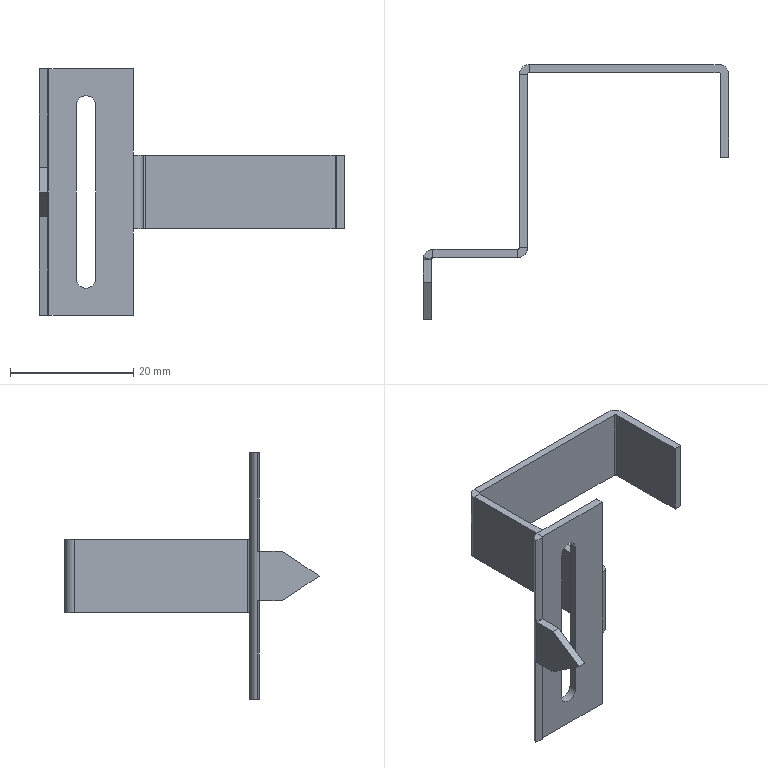Part | NX | 1 solid | 48 faces | box 49.6 x 41.3 x 40 mm | volume 1923 mm3 | plane 37 | cylinder 11 | commonest cylinder face diameters 3.2 x7 0.6 x4
STEP:
#1=CARTESIAN_POINT('',(6.,-1.3,35.6));
#2=VERTEX_POINT('',#1);
#3=CARTESIAN_POINT('',(7.6,-1.3,34.));
#4=VERTEX_POINT('',#3);
#5=CARTESIAN_POINT('',(6.,-1.3,34.));
#6=DIRECTION('',(0.,1.,0.));
#7=DIRECTION('',(0.,0.,1.));
#8=AXIS2_PLACEMENT_3D('',#5,#6,#7);
#9=CIRCLE('',#8,1.6);
#10=EDGE_CURVE('',#2,#4,#9,.T.);
#11=ORIENTED_EDGE('',*,*,#10,.F.);
#12=CARTESIAN_POINT('',(6.,0.,35.6));
#13=VERTEX_POINT('',#12);
#14=CARTESIAN_POINT('',(6.,-10.,35.6));
#15=DIRECTION('',(0.,1.,0.));
#16=VECTOR('',#15,1.);
#17=LINE('',#14,#16);
#18=EDGE_CURVE('',#2,#13,#17,.T.);
#19=ORIENTED_EDGE('',*,*,#18,.T.);
#20=CARTESIAN_POINT('',(7.6,0.,34.));
#21=VERTEX_POINT('',#20);
#22=CARTESIAN_POINT('',(6.,0.,34.));
#23=DIRECTION('',(0.,1.,0.));
#24=DIRECTION('',(0.,0.,1.));
#25=AXIS2_PLACEMENT_3D('',#22,#23,#24);
#26=CIRCLE('',#25,1.6);
#27=EDGE_CURVE('',#13,#21,#26,.T.);
#28=ORIENTED_EDGE('',*,*,#27,.T.);
#29=CARTESIAN_POINT('',(7.6,-10.,34.));
#30=DIRECTION('',(0.,1.,0.));
#31=VECTOR('',#30,1.);
#32=LINE('',#29,#31);
#33=EDGE_CURVE('',#4,#21,#32,.T.);
#34=ORIENTED_EDGE('',*,*,#33,.F.);
#35=EDGE_LOOP('',(#11,#19,#28,#34));
#36=FACE_OUTER_BOUND('',#35,.T.);
#37=CARTESIAN_POINT('',(6.,-10.,34.));
#38=DIRECTION('',(0.,1.,0.));
#39=DIRECTION('',(0.,0.,1.));
#40=AXIS2_PLACEMENT_3D('',#37,#38,#39);
#41=CYLINDRICAL_SURFACE('',#40,1.6);
#42=ADVANCED_FACE('',(#36),#41,.F.);
#43=CARTESIAN_POINT('',(-1.6,-5.3,16.));
#44=VERTEX_POINT('',#43);
#45=CARTESIAN_POINT('',(-1.6,-11.3,20.));
#46=VERTEX_POINT('',#45);
#47=CARTESIAN_POINT('',(-1.6,5.754,8.631));
#48=DIRECTION('',(0.,-0.8321,0.5547));
#49=VECTOR('',#48,1.);
#50=LINE('',#47,#49);
#51=EDGE_CURVE('',#44,#46,#50,.T.);
#52=ORIENTED_EDGE('',*,*,#51,.T.);
#53=CARTESIAN_POINT('',(-1.6,-5.3,24.));
#54=VERTEX_POINT('',#53);
#55=CARTESIAN_POINT('',(-1.6,-12.708,19.062));
#56=DIRECTION('',(0.,0.8321,0.5547));
#57=VECTOR('',#56,1.);
#58=LINE('',#55,#57);
#59=EDGE_CURVE('',#46,#54,#58,.T.);
#60=ORIENTED_EDGE('',*,*,#59,.T.);
#61=CARTESIAN_POINT('',(-1.6,-1.6,24.));
#62=VERTEX_POINT('',#61);
#63=CARTESIAN_POINT('',(-1.6,0.,24.));
#64=DIRECTION('',(0.,-1.,0.));
#65=VECTOR('',#64,1.);
#66=LINE('',#63,#65);
#67=EDGE_CURVE('',#62,#54,#66,.T.);
#68=ORIENTED_EDGE('',*,*,#67,.F.);
#69=CARTESIAN_POINT('',(-1.6,-1.6,16.));
#70=VERTEX_POINT('',#69);
#71=CARTESIAN_POINT('',(-1.6,-1.6,40.));
#72=DIRECTION('',(0.,0.,1.));
#73=VECTOR('',#72,1.);
#74=LINE('',#71,#73);
#75=EDGE_CURVE('',#70,#62,#74,.T.);
#76=ORIENTED_EDGE('',*,*,#75,.F.);
#77=CARTESIAN_POINT('',(-1.6,-1.3,16.));
#78=DIRECTION('',(0.,-1.,0.));
#79=VECTOR('',#78,1.);
#80=LINE('',#77,#79);
#81=EDGE_CURVE('',#70,#44,#80,.T.);
#82=ORIENTED_EDGE('',*,*,#81,.T.);
#83=EDGE_LOOP('',(#52,#60,#68,#76,#82));
#84=FACE_OUTER_BOUND('',#83,.T.);
#85=CARTESIAN_POINT('',(-1.6,0.,0.));
#86=DIRECTION('',(1.,0.,0.));
#87=DIRECTION('',(0.,1.,0.));
#88=AXIS2_PLACEMENT_3D('',#85,#86,#87);
#89=PLANE('',#88);
#90=ADVANCED_FACE('',(#84),#89,.F.);
#91=CARTESIAN_POINT('',(-0.3,-11.3,20.));
#92=VERTEX_POINT('',#91);
#93=CARTESIAN_POINT('',(-0.3,-5.3,24.));
#94=VERTEX_POINT('',#93);
#95=CARTESIAN_POINT('',(-0.3,-12.708,19.062));
#96=DIRECTION('',(0.,0.8321,0.5547));
#97=VECTOR('',#96,1.);
#98=LINE('',#95,#97);
#99=EDGE_CURVE('',#92,#94,#98,.T.);
#100=ORIENTED_EDGE('',*,*,#99,.F.);
#101=CARTESIAN_POINT('',(-0.3,-5.3,16.));
#102=VERTEX_POINT('',#101);
#103=CARTESIAN_POINT('',(-0.3,5.754,8.631));
#104=DIRECTION('',(0.,-0.8321,0.5547));
#105=VECTOR('',#104,1.);
#106=LINE('',#103,#105);
#107=EDGE_CURVE('',#102,#92,#106,.T.);
#108=ORIENTED_EDGE('',*,*,#107,.F.);
#109=CARTESIAN_POINT('',(-0.3,-1.6,16.));
#110=VERTEX_POINT('',#109);
#111=CARTESIAN_POINT('',(-0.3,0.,16.));
#112=DIRECTION('',(0.,-1.,0.));
#113=VECTOR('',#112,1.);
#114=LINE('',#111,#113);
#115=EDGE_CURVE('',#110,#102,#114,.T.);
#116=ORIENTED_EDGE('',*,*,#115,.F.);
#117=CARTESIAN_POINT('',(-0.3,-1.6,24.));
#118=VERTEX_POINT('',#117);
#119=CARTESIAN_POINT('',(-0.3,-1.6,40.));
#120=DIRECTION('',(0.,0.,-1.));
#121=VECTOR('',#120,1.);
#122=LINE('',#119,#121);
#123=EDGE_CURVE('',#118,#110,#122,.T.);
#124=ORIENTED_EDGE('',*,*,#123,.F.);
#125=CARTESIAN_POINT('',(-0.3,-1.3,24.));
#126=DIRECTION('',(0.,-1.,0.));
#127=VECTOR('',#126,1.);
#128=LINE('',#125,#127);
#129=EDGE_CURVE('',#118,#94,#128,.T.);
#130=ORIENTED_EDGE('',*,*,#129,.T.);
#131=EDGE_LOOP('',(#100,#108,#116,#124,#130));
#132=FACE_OUTER_BOUND('',#131,.T.);
#133=CARTESIAN_POINT('',(-0.3,0.,0.));
#134=DIRECTION('',(1.,0.,0.));
#135=DIRECTION('',(0.,1.,0.));
#136=AXIS2_PLACEMENT_3D('',#133,#134,#135);
#137=PLANE('',#136);
#138=ADVANCED_FACE('',(#132),#137,.T.);
#139=ORIENTED_EDGE('',*,*,#115,.T.);
#140=CARTESIAN_POINT('',(-1.6,-5.3,16.));
#141=DIRECTION('',(1.,0.,0.));
#142=VECTOR('',#141,1.);
#143=LINE('',#140,#142);
#144=EDGE_CURVE('',#44,#102,#143,.T.);
#145=ORIENTED_EDGE('',*,*,#144,.F.);
#146=ORIENTED_EDGE('',*,*,#81,.F.);
#147=CARTESIAN_POINT('',(-1.6,-1.6,16.));
#148=DIRECTION('',(1.,0.,0.));
#149=VECTOR('',#148,1.);
#150=LINE('',#147,#149);
#151=EDGE_CURVE('',#70,#110,#150,.T.);
#152=ORIENTED_EDGE('',*,*,#151,.T.);
#153=EDGE_LOOP('',(#139,#145,#146,#152));
#154=FACE_OUTER_BOUND('',#153,.T.);
#155=CARTESIAN_POINT('',(-1.6,-1.3,16.));
#156=DIRECTION('',(0.,0.,1.));
#157=DIRECTION('',(0.,-1.,0.));
#158=AXIS2_PLACEMENT_3D('',#155,#156,#157);
#159=PLANE('',#158);
#160=ADVANCED_FACE('',(#154),#159,.F.);
#161=ORIENTED_EDGE('',*,*,#67,.T.);
#162=CARTESIAN_POINT('',(-1.6,-5.3,24.));
#163=DIRECTION('',(1.,0.,0.));
#164=VECTOR('',#163,1.);
#165=LINE('',#162,#164);
#166=EDGE_CURVE('',#54,#94,#165,.T.);
#167=ORIENTED_EDGE('',*,*,#166,.T.);
#168=ORIENTED_EDGE('',*,*,#129,.F.);
#169=CARTESIAN_POINT('',(-0.3,-1.6,24.));
#170=DIRECTION('',(-1.,0.,0.));
#171=VECTOR('',#170,1.);
#172=LINE('',#169,#171);
#173=EDGE_CURVE('',#118,#62,#172,.T.);
#174=ORIENTED_EDGE('',*,*,#173,.T.);
#175=EDGE_LOOP('',(#161,#167,#168,#174));
#176=FACE_OUTER_BOUND('',#175,.T.);
#177=CARTESIAN_POINT('',(-0.3,-1.3,24.));
#178=DIRECTION('',(0.,0.,1.));
#179=DIRECTION('',(0.,-1.,0.));
#180=AXIS2_PLACEMENT_3D('',#177,#178,#179);
#181=PLANE('',#180);
#182=ADVANCED_FACE('',(#176),#181,.T.);
#183=CARTESIAN_POINT('',(-1.572,-1.3,24.));
#184=VERTEX_POINT('',#183);
#185=CARTESIAN_POINT('',(0.,-1.6,24.));
#186=DIRECTION('',(0.,0.,1.));
#187=DIRECTION('',(-1.,0.,0.));
#188=AXIS2_PLACEMENT_3D('',#185,#186,#187);
#189=CIRCLE('',#188,1.6);
#190=EDGE_CURVE('',#184,#62,#189,.T.);
#191=ORIENTED_EDGE('',*,*,#190,.F.);
#192=CARTESIAN_POINT('',(-1.572,-1.3,40.));
#193=VERTEX_POINT('',#192);
#194=CARTESIAN_POINT('',(-1.572,-1.3,0.));
#195=DIRECTION('',(0.,0.,-1.));
#196=VECTOR('',#195,1.);
#197=LINE('',#194,#196);
#198=EDGE_CURVE('',#193,#184,#197,.T.);
#199=ORIENTED_EDGE('',*,*,#198,.F.);
#200=CARTESIAN_POINT('',(0.,0.,40.));
#201=VERTEX_POINT('',#200);
#202=CARTESIAN_POINT('',(0.,-1.6,40.));
#203=DIRECTION('',(0.,0.,1.));
#204=DIRECTION('',(-1.,0.,0.));
#205=AXIS2_PLACEMENT_3D('',#202,#203,#204);
#206=CIRCLE('',#205,1.6);
#207=EDGE_CURVE('',#201,#193,#206,.T.);
#208=ORIENTED_EDGE('',*,*,#207,.F.);
#209=CARTESIAN_POINT('',(0.,0.,0.));
#210=VERTEX_POINT('',#209);
#211=CARTESIAN_POINT('',(0.,0.,40.));
#212=DIRECTION('',(0.,0.,-1.));
#213=VECTOR('',#212,1.);
#214=LINE('',#211,#213);
#215=EDGE_CURVE('',#201,#210,#214,.T.);
#216=ORIENTED_EDGE('',*,*,#215,.T.);
#217=CARTESIAN_POINT('',(-1.572,-1.3,0.));
#218=VERTEX_POINT('',#217);
#219=CARTESIAN_POINT('',(0.,-1.6,0.));
#220=DIRECTION('',(0.,0.,-1.));
#221=DIRECTION('',(-1.,0.,0.));
#222=AXIS2_PLACEMENT_3D('',#219,#220,#221);
#223=CIRCLE('',#222,1.6);
#224=EDGE_CURVE('',#218,#210,#223,.T.);
#225=ORIENTED_EDGE('',*,*,#224,.F.);
#226=CARTESIAN_POINT('',(-1.572,-1.3,16.));
#227=VERTEX_POINT('',#226);
#228=CARTESIAN_POINT('',(-1.572,-1.3,0.));
#229=DIRECTION('',(0.,0.,-1.));
#230=VECTOR('',#229,1.);
#231=LINE('',#228,#230);
#232=EDGE_CURVE('',#227,#218,#231,.T.);
#233=ORIENTED_EDGE('',*,*,#232,.F.);
#234=CARTESIAN_POINT('',(0.,-1.6,16.));
#235=DIRECTION('',(0.,0.,-1.));
#236=DIRECTION('',(1.,0.,0.));
#237=AXIS2_PLACEMENT_3D('',#234,#235,#236);
#238=CIRCLE('',#237,1.6);
#239=EDGE_CURVE('',#70,#227,#238,.T.);
#240=ORIENTED_EDGE('',*,*,#239,.F.);
#241=ORIENTED_EDGE('',*,*,#75,.T.);
#242=EDGE_LOOP('',(#191,#199,#208,#216,#225,#233,#240,#241));
#243=FACE_OUTER_BOUND('',#242,.T.);
#244=CARTESIAN_POINT('',(0.,-1.6,0.));
#245=DIRECTION('',(0.,0.,-1.));
#246=DIRECTION('',(-1.,0.,0.));
#247=AXIS2_PLACEMENT_3D('',#244,#245,#246);
#248=CYLINDRICAL_SURFACE('',#247,1.6);
#249=ADVANCED_FACE('',(#243),#248,.T.);
#250=CARTESIAN_POINT('',(-0.2947,-1.544,40.));
#251=VERTEX_POINT('',#250);
#252=CARTESIAN_POINT('',(-0.2947,-1.544,24.));
#253=VERTEX_POINT('',#252);
#254=CARTESIAN_POINT('',(-0.2947,-1.544,0.));
#255=DIRECTION('',(0.,0.,-1.));
#256=VECTOR('',#255,1.);
#257=LINE('',#254,#256);
#258=EDGE_CURVE('',#251,#253,#257,.T.);
#259=ORIENTED_EDGE('',*,*,#258,.T.);
#260=CARTESIAN_POINT('',(0.,-1.6,24.));
#261=DIRECTION('',(0.,0.,1.));
#262=DIRECTION('',(-1.,0.,0.));
#263=AXIS2_PLACEMENT_3D('',#260,#261,#262);
#264=CIRCLE('',#263,0.3);
#265=EDGE_CURVE('',#253,#118,#264,.T.);
#266=ORIENTED_EDGE('',*,*,#265,.T.);
#267=ORIENTED_EDGE('',*,*,#123,.T.);
#268=CARTESIAN_POINT('',(-0.2947,-1.544,16.));
#269=VERTEX_POINT('',#268);
#270=CARTESIAN_POINT('',(0.,-1.6,16.));
#271=DIRECTION('',(0.,0.,-1.));
#272=DIRECTION('',(-1.,0.,0.));
#273=AXIS2_PLACEMENT_3D('',#270,#271,#272);
#274=CIRCLE('',#273,0.3);
#275=EDGE_CURVE('',#110,#269,#274,.T.);
#276=ORIENTED_EDGE('',*,*,#275,.T.);
#277=CARTESIAN_POINT('',(-0.2947,-1.544,0.));
#278=VERTEX_POINT('',#277);
#279=CARTESIAN_POINT('',(-0.2947,-1.544,0.));
#280=DIRECTION('',(0.,0.,-1.));
#281=VECTOR('',#280,1.);
#282=LINE('',#279,#281);
#283=EDGE_CURVE('',#269,#278,#282,.T.);
#284=ORIENTED_EDGE('',*,*,#283,.T.);
#285=CARTESIAN_POINT('',(0.,-1.3,0.));
#286=VERTEX_POINT('',#285);
#287=CARTESIAN_POINT('',(0.,-1.6,0.));
#288=DIRECTION('',(0.,0.,-1.));
#289=DIRECTION('',(-1.,0.,0.));
#290=AXIS2_PLACEMENT_3D('',#287,#288,#289);
#291=CIRCLE('',#290,0.3);
#292=EDGE_CURVE('',#278,#286,#291,.T.);
#293=ORIENTED_EDGE('',*,*,#292,.T.);
#294=CARTESIAN_POINT('',(0.,-1.3,40.));
#295=VERTEX_POINT('',#294);
#296=CARTESIAN_POINT('',(0.,-1.3,40.));
#297=DIRECTION('',(0.,0.,-1.));
#298=VECTOR('',#297,1.);
#299=LINE('',#296,#298);
#300=EDGE_CURVE('',#295,#286,#299,.T.);
#301=ORIENTED_EDGE('',*,*,#300,.F.);
#302=CARTESIAN_POINT('',(0.,-1.6,40.));
#303=DIRECTION('',(0.,0.,1.));
#304=DIRECTION('',(-1.,0.,0.));
#305=AXIS2_PLACEMENT_3D('',#302,#303,#304);
#306=CIRCLE('',#305,0.3);
#307=EDGE_CURVE('',#295,#251,#306,.T.);
#308=ORIENTED_EDGE('',*,*,#307,.T.);
#309=EDGE_LOOP('',(#259,#266,#267,#276,#284,#293,#301,#308));
#310=FACE_OUTER_BOUND('',#309,.T.);
#311=CARTESIAN_POINT('',(0.,-1.6,0.));
#312=DIRECTION('',(0.,0.,-1.));
#313=DIRECTION('',(-1.,0.,0.));
#314=AXIS2_PLACEMENT_3D('',#311,#312,#313);
#315=CYLINDRICAL_SURFACE('',#314,0.3);
#316=ADVANCED_FACE('',(#310),#315,.F.);
#317=ORIENTED_EDGE('',*,*,#207,.T.);
#318=CARTESIAN_POINT('',(-1.572,-1.3,40.));
#319=DIRECTION('',(0.9823,-0.1875,0.));
#320=VECTOR('',#319,1.);
#321=LINE('',#318,#320);
#322=EDGE_CURVE('',#193,#251,#321,.T.);
#323=ORIENTED_EDGE('',*,*,#322,.T.);
#324=ORIENTED_EDGE('',*,*,#307,.F.);
#325=CARTESIAN_POINT('',(0.,-1.3,40.));
#326=DIRECTION('',(0.,1.,0.));
#327=VECTOR('',#326,1.);
#328=LINE('',#325,#327);
#329=EDGE_CURVE('',#295,#201,#328,.T.);
#330=ORIENTED_EDGE('',*,*,#329,.T.);
#331=EDGE_LOOP('',(#317,#323,#324,#330));
#332=FACE_OUTER_BOUND('',#331,.T.);
#333=CARTESIAN_POINT('',(0.,-1.6,40.));
#334=DIRECTION('',(0.,0.,1.));
#335=DIRECTION('',(1.,0.,0.));
#336=AXIS2_PLACEMENT_3D('',#333,#334,#335);
#337=PLANE('',#336);
#338=ADVANCED_FACE('',(#332),#337,.T.);
#339=ORIENTED_EDGE('',*,*,#292,.F.);
#340=CARTESIAN_POINT('',(-1.572,-1.3,0.));
#341=DIRECTION('',(0.9823,-0.1875,0.));
#342=VECTOR('',#341,1.);
#343=LINE('',#340,#342);
#344=EDGE_CURVE('',#218,#278,#343,.T.);
#345=ORIENTED_EDGE('',*,*,#344,.F.);
#346=ORIENTED_EDGE('',*,*,#224,.T.);
#347=CARTESIAN_POINT('',(0.,-1.3,0.));
#348=DIRECTION('',(0.,1.,0.));
#349=VECTOR('',#348,1.);
#350=LINE('',#347,#349);
#351=EDGE_CURVE('',#286,#210,#350,.T.);
#352=ORIENTED_EDGE('',*,*,#351,.F.);
#353=EDGE_LOOP('',(#339,#345,#346,#352));
#354=FACE_OUTER_BOUND('',#353,.T.);
#355=CARTESIAN_POINT('',(0.,-1.6,0.));
#356=DIRECTION('',(0.,0.,1.));
#357=DIRECTION('',(1.,0.,0.));
#358=AXIS2_PLACEMENT_3D('',#355,#356,#357);
#359=PLANE('',#358);
#360=ADVANCED_FACE('',(#354),#359,.F.);
#361=CARTESIAN_POINT('',(14.,28.4,26.));
#362=VERTEX_POINT('',#361);
#363=CARTESIAN_POINT('',(14.,0.3,26.));
#364=VERTEX_POINT('',#363);
#365=CARTESIAN_POINT('',(14.,0.,26.));
#366=DIRECTION('',(0.,-1.,0.));
#367=VECTOR('',#366,1.);
#368=LINE('',#365,#367);
#369=EDGE_CURVE('',#362,#364,#368,.T.);
#370=ORIENTED_EDGE('',*,*,#369,.T.);
#371=CARTESIAN_POINT('',(15.3,0.3,26.));
#372=VERTEX_POINT('',#371);
#373=CARTESIAN_POINT('',(14.,0.3,26.));
#374=DIRECTION('',(1.,0.,0.));
#375=VECTOR('',#374,1.);
#376=LINE('',#373,#375);
#377=EDGE_CURVE('',#364,#372,#376,.T.);
#378=ORIENTED_EDGE('',*,*,#377,.T.);
#379=CARTESIAN_POINT('',(15.3,28.4,26.));
#380=VERTEX_POINT('',#379);
#381=CARTESIAN_POINT('',(15.3,0.,26.));
#382=DIRECTION('',(0.,-1.,0.));
#383=VECTOR('',#382,1.);
#384=LINE('',#381,#383);
#385=EDGE_CURVE('',#380,#372,#384,.T.);
#386=ORIENTED_EDGE('',*,*,#385,.F.);
#387=CARTESIAN_POINT('',(15.3,28.4,26.));
#388=DIRECTION('',(-1.,0.,0.));
#389=VECTOR('',#388,1.);
#390=LINE('',#387,#389);
#391=EDGE_CURVE('',#380,#362,#390,.T.);
#392=ORIENTED_EDGE('',*,*,#391,.T.);
#393=EDGE_LOOP('',(#370,#378,#386,#392));
#394=FACE_OUTER_BOUND('',#393,.T.);
#395=CARTESIAN_POINT('',(13.7,-1.3,26.));
#396=DIRECTION('',(0.,0.,-1.));
#397=DIRECTION('',(-1.,0.,0.));
#398=AXIS2_PLACEMENT_3D('',#395,#396,#397);
#399=PLANE('',#398);
#400=ADVANCED_FACE('',(#394),#399,.F.);
#401=ORIENTED_EDGE('',*,*,#377,.F.);
#402=CARTESIAN_POINT('',(13.7,0.,26.));
#403=VERTEX_POINT('',#402);
#404=CARTESIAN_POINT('',(13.7,0.3,26.));
#405=DIRECTION('',(0.,0.,-1.));
#406=DIRECTION('',(-1.,0.,0.));
#407=AXIS2_PLACEMENT_3D('',#404,#405,#406);
#408=CIRCLE('',#407,0.3);
#409=EDGE_CURVE('',#364,#403,#408,.T.);
#410=ORIENTED_EDGE('',*,*,#409,.T.);
#411=CARTESIAN_POINT('',(13.7,-1.3,26.));
#412=VERTEX_POINT('',#411);
#413=CARTESIAN_POINT('',(13.7,-1.3,26.));
#414=DIRECTION('',(0.,1.,0.));
#415=VECTOR('',#414,1.);
#416=LINE('',#413,#415);
#417=EDGE_CURVE('',#412,#403,#416,.T.);
#418=ORIENTED_EDGE('',*,*,#417,.F.);
#419=CARTESIAN_POINT('',(13.7,0.3,26.));
#420=DIRECTION('',(0.,0.,-1.));
#421=DIRECTION('',(-1.,0.,0.));
#422=AXIS2_PLACEMENT_3D('',#419,#420,#421);
#423=CIRCLE('',#422,1.6);
#424=EDGE_CURVE('',#372,#412,#423,.T.);
#425=ORIENTED_EDGE('',*,*,#424,.F.);
#426=EDGE_LOOP('',(#401,#410,#418,#425));
#427=FACE_OUTER_BOUND('',#426,.T.);
#428=CARTESIAN_POINT('',(13.7,-1.3,26.));
#429=DIRECTION('',(0.,0.,-1.));
#430=DIRECTION('',(-1.,0.,0.));
#431=AXIS2_PLACEMENT_3D('',#428,#429,#430);
#432=PLANE('',#431);
#433=ADVANCED_FACE('',(#427),#432,.F.);
#434=CARTESIAN_POINT('',(46.4,30.,26.));
#435=VERTEX_POINT('',#434);
#436=CARTESIAN_POINT('',(15.6,30.,26.));
#437=VERTEX_POINT('',#436);
#438=CARTESIAN_POINT('',(13.7,30.,26.));
#439=DIRECTION('',(-1.,0.,0.));
#440=VECTOR('',#439,1.);
#441=LINE('',#438,#440);
#442=EDGE_CURVE('',#435,#437,#441,.T.);
#443=ORIENTED_EDGE('',*,*,#442,.T.);
#444=CARTESIAN_POINT('',(15.6,28.7,26.));
#445=VERTEX_POINT('',#444);
#446=CARTESIAN_POINT('',(15.6,30.,26.));
#447=DIRECTION('',(0.,-1.,0.));
#448=VECTOR('',#447,1.);
#449=LINE('',#446,#448);
#450=EDGE_CURVE('',#437,#445,#449,.T.);
#451=ORIENTED_EDGE('',*,*,#450,.T.);
#452=CARTESIAN_POINT('',(46.4,28.7,26.));
#453=VERTEX_POINT('',#452);
#454=CARTESIAN_POINT('',(14.,28.7,26.));
#455=DIRECTION('',(-1.,0.,0.));
#456=VECTOR('',#455,1.);
#457=LINE('',#454,#456);
#458=EDGE_CURVE('',#453,#445,#457,.T.);
#459=ORIENTED_EDGE('',*,*,#458,.F.);
#460=CARTESIAN_POINT('',(46.7,28.4,26.));
#461=VERTEX_POINT('',#460);
#462=CARTESIAN_POINT('',(46.4,28.4,26.));
#463=DIRECTION('',(0.,0.,1.));
#464=DIRECTION('',(-1.,0.,0.));
#465=AXIS2_PLACEMENT_3D('',#462,#463,#464);
#466=CIRCLE('',#465,0.3);
#467=EDGE_CURVE('',#461,#453,#466,.T.);
#468=ORIENTED_EDGE('',*,*,#467,.F.);
#469=CARTESIAN_POINT('',(46.7,15.,26.));
#470=VERTEX_POINT('',#469);
#471=CARTESIAN_POINT('',(46.7,30.,26.));
#472=DIRECTION('',(0.,1.,0.));
#473=VECTOR('',#472,1.);
#474=LINE('',#471,#473);
#475=EDGE_CURVE('',#470,#461,#474,.T.);
#476=ORIENTED_EDGE('',*,*,#475,.F.);
#477=CARTESIAN_POINT('',(48.,15.,26.));
#478=VERTEX_POINT('',#477);
#479=CARTESIAN_POINT('',(48.,15.,26.));
#480=DIRECTION('',(1.,0.,0.));
#481=VECTOR('',#480,1.);
#482=LINE('',#479,#481);
#483=EDGE_CURVE('',#470,#478,#482,.T.);
#484=ORIENTED_EDGE('',*,*,#483,.T.);
#485=CARTESIAN_POINT('',(48.,28.4,26.));
#486=VERTEX_POINT('',#485);
#487=CARTESIAN_POINT('',(48.,30.,26.));
#488=DIRECTION('',(0.,1.,0.));
#489=VECTOR('',#488,1.);
#490=LINE('',#487,#489);
#491=EDGE_CURVE('',#478,#486,#490,.T.);
#492=ORIENTED_EDGE('',*,*,#491,.T.);
#493=CARTESIAN_POINT('',(46.4,28.4,26.));
#494=DIRECTION('',(0.,0.,1.));
#495=DIRECTION('',(-1.,0.,0.));
#496=AXIS2_PLACEMENT_3D('',#493,#494,#495);
#497=CIRCLE('',#496,1.6);
#498=EDGE_CURVE('',#486,#435,#497,.T.);
#499=ORIENTED_EDGE('',*,*,#498,.T.);
#500=EDGE_LOOP('',(#443,#451,#459,#468,#476,#484,#492,#499));
#501=FACE_OUTER_BOUND('',#500,.T.);
#502=CARTESIAN_POINT('',(13.7,-1.3,26.));
#503=DIRECTION('',(0.,0.,-1.));
#504=DIRECTION('',(-1.,0.,0.));
#505=AXIS2_PLACEMENT_3D('',#502,#503,#504);
#506=PLANE('',#505);
#507=ADVANCED_FACE('',(#501),#506,.F.);
#508=CARTESIAN_POINT('',(15.3,0.3,14.));
#509=VERTEX_POINT('',#508);
#510=CARTESIAN_POINT('',(15.3,28.4,14.));
#511=VERTEX_POINT('',#510);
#512=CARTESIAN_POINT('',(15.3,0.,14.));
#513=DIRECTION('',(0.,1.,0.));
#514=VECTOR('',#513,1.);
#515=LINE('',#512,#514);
#516=EDGE_CURVE('',#509,#511,#515,.T.);
#517=ORIENTED_EDGE('',*,*,#516,.F.);
#518=CARTESIAN_POINT('',(14.,0.3,14.));
#519=VERTEX_POINT('',#518);
#520=CARTESIAN_POINT('',(15.3,0.3,14.));
#521=DIRECTION('',(-1.,0.,0.));
#522=VECTOR('',#521,1.);
#523=LINE('',#520,#522);
#524=EDGE_CURVE('',#509,#519,#523,.T.);
#525=ORIENTED_EDGE('',*,*,#524,.T.);
#526=CARTESIAN_POINT('',(14.,28.4,14.));
#527=VERTEX_POINT('',#526);
#528=CARTESIAN_POINT('',(14.,0.,14.));
#529=DIRECTION('',(0.,1.,0.));
#530=VECTOR('',#529,1.);
#531=LINE('',#528,#530);
#532=EDGE_CURVE('',#519,#527,#531,.T.);
#533=ORIENTED_EDGE('',*,*,#532,.T.);
#534=CARTESIAN_POINT('',(14.,28.4,14.));
#535=DIRECTION('',(1.,0.,0.));
#536=VECTOR('',#535,1.);
#537=LINE('',#534,#536);
#538=EDGE_CURVE('',#527,#511,#537,.T.);
#539=ORIENTED_EDGE('',*,*,#538,.T.);
#540=EDGE_LOOP('',(#517,#525,#533,#539));
#541=FACE_OUTER_BOUND('',#540,.T.);
#542=CARTESIAN_POINT('',(13.7,-1.3,14.));
#543=DIRECTION('',(0.,0.,1.));
#544=DIRECTION('',(1.,0.,0.));
#545=AXIS2_PLACEMENT_3D('',#542,#543,#544);
#546=PLANE('',#545);
#547=ADVANCED_FACE('',(#541),#546,.F.);
#548=CARTESIAN_POINT('',(46.7,28.4,14.));
#549=VERTEX_POINT('',#548);
#550=CARTESIAN_POINT('',(46.7,15.,14.));
#551=VERTEX_POINT('',#550);
#552=CARTESIAN_POINT('',(46.7,30.,14.));
#553=DIRECTION('',(0.,-1.,0.));
#554=VECTOR('',#553,1.);
#555=LINE('',#552,#554);
#556=EDGE_CURVE('',#549,#551,#555,.T.);
#557=ORIENTED_EDGE('',*,*,#556,.F.);
#558=CARTESIAN_POINT('',(48.,28.4,14.));
#559=VERTEX_POINT('',#558);
#560=CARTESIAN_POINT('',(46.7,28.4,14.));
#561=DIRECTION('',(1.,0.,0.));
#562=VECTOR('',#561,1.);
#563=LINE('',#560,#562);
#564=EDGE_CURVE('',#549,#559,#563,.T.);
#565=ORIENTED_EDGE('',*,*,#564,.T.);
#566=CARTESIAN_POINT('',(48.,15.,14.));
#567=VERTEX_POINT('',#566);
#568=CARTESIAN_POINT('',(48.,30.,14.));
#569=DIRECTION('',(0.,-1.,0.));
#570=VECTOR('',#569,1.);
#571=LINE('',#568,#570);
#572=EDGE_CURVE('',#559,#567,#571,.T.);
#573=ORIENTED_EDGE('',*,*,#572,.T.);
#574=CARTESIAN_POINT('',(48.,15.,14.));
#575=DIRECTION('',(-1.,0.,0.));
#576=VECTOR('',#575,1.);
#577=LINE('',#574,#576);
#578=EDGE_CURVE('',#567,#551,#577,.T.);
#579=ORIENTED_EDGE('',*,*,#578,.T.);
#580=EDGE_LOOP('',(#557,#565,#573,#579));
#581=FACE_OUTER_BOUND('',#580,.T.);
#582=CARTESIAN_POINT('',(13.7,-1.3,14.));
#583=DIRECTION('',(0.,0.,1.));
#584=DIRECTION('',(1.,0.,0.));
#585=AXIS2_PLACEMENT_3D('',#582,#583,#584);
#586=PLANE('',#585);
#587=ADVANCED_FACE('',(#581),#586,.F.);
#588=CARTESIAN_POINT('',(15.6,30.,14.));
#589=VERTEX_POINT('',#588);
#590=CARTESIAN_POINT('',(46.4,30.,14.));
#591=VERTEX_POINT('',#590);
#592=CARTESIAN_POINT('',(13.7,30.,14.));
#593=DIRECTION('',(1.,0.,0.));
#594=VECTOR('',#593,1.);
#595=LINE('',#592,#594);
#596=EDGE_CURVE('',#589,#591,#595,.T.);
#597=ORIENTED_EDGE('',*,*,#596,.T.);
#598=CARTESIAN_POINT('',(46.4,28.7,14.));
#599=VERTEX_POINT('',#598);
#600=CARTESIAN_POINT('',(46.4,30.,14.));
#601=DIRECTION('',(0.,-1.,0.));
#602=VECTOR('',#601,1.);
#603=LINE('',#600,#602);
#604=EDGE_CURVE('',#591,#599,#603,.T.);
#605=ORIENTED_EDGE('',*,*,#604,.T.);
#606=CARTESIAN_POINT('',(15.6,28.7,14.));
#607=VERTEX_POINT('',#606);
#608=CARTESIAN_POINT('',(14.,28.7,14.));
#609=DIRECTION('',(1.,0.,0.));
#610=VECTOR('',#609,1.);
#611=LINE('',#608,#610);
#612=EDGE_CURVE('',#607,#599,#611,.T.);
#613=ORIENTED_EDGE('',*,*,#612,.F.);
#614=CARTESIAN_POINT('',(15.6,28.7,14.));
#615=DIRECTION('',(0.,1.,0.));
#616=VECTOR('',#615,1.);
#617=LINE('',#614,#616);
#618=EDGE_CURVE('',#607,#589,#617,.T.);
#619=ORIENTED_EDGE('',*,*,#618,.T.);
#620=EDGE_LOOP('',(#597,#605,#613,#619));
#621=FACE_OUTER_BOUND('',#620,.T.);
#622=CARTESIAN_POINT('',(13.7,-1.3,14.));
#623=DIRECTION('',(0.,0.,1.));
#624=DIRECTION('',(1.,0.,0.));
#625=AXIS2_PLACEMENT_3D('',#622,#623,#624);
#626=PLANE('',#625);
#627=ADVANCED_FACE('',(#621),#626,.F.);
#628=ORIENTED_EDGE('',*,*,#564,.F.);
#629=CARTESIAN_POINT('',(46.4,28.4,14.));
#630=DIRECTION('',(0.,0.,-1.));
#631=DIRECTION('',(1.,0.,0.));
#632=AXIS2_PLACEMENT_3D('',#629,#630,#631);
#633=CIRCLE('',#632,0.3);
#634=EDGE_CURVE('',#599,#549,#633,.T.);
#635=ORIENTED_EDGE('',*,*,#634,.F.);
#636=ORIENTED_EDGE('',*,*,#604,.F.);
#637=CARTESIAN_POINT('',(46.4,28.4,14.));
#638=DIRECTION('',(0.,0.,-1.));
#639=DIRECTION('',(1.,0.,0.));
#640=AXIS2_PLACEMENT_3D('',#637,#638,#639);
#641=CIRCLE('',#640,1.6);
#642=EDGE_CURVE('',#591,#559,#641,.T.);
#643=ORIENTED_EDGE('',*,*,#642,.T.);
#644=EDGE_LOOP('',(#628,#635,#636,#643));
#645=FACE_OUTER_BOUND('',#644,.T.);
#646=CARTESIAN_POINT('',(13.7,-1.3,14.));
#647=DIRECTION('',(0.,0.,1.));
#648=DIRECTION('',(1.,0.,0.));
#649=AXIS2_PLACEMENT_3D('',#646,#647,#648);
#650=PLANE('',#649);
#651=ADVANCED_FACE('',(#645),#650,.F.);
#652=ORIENTED_EDGE('',*,*,#524,.F.);
#653=CARTESIAN_POINT('',(13.7,-1.3,14.));
#654=VERTEX_POINT('',#653);
#655=CARTESIAN_POINT('',(13.7,0.3,14.));
#656=DIRECTION('',(0.,0.,1.));
#657=DIRECTION('',(1.,0.,0.));
#658=AXIS2_PLACEMENT_3D('',#655,#656,#657);
#659=CIRCLE('',#658,1.6);
#660=EDGE_CURVE('',#654,#509,#659,.T.);
#661=ORIENTED_EDGE('',*,*,#660,.F.);
#662=CARTESIAN_POINT('',(13.7,0.,14.));
#663=VERTEX_POINT('',#662);
#664=CARTESIAN_POINT('',(13.7,-1.3,14.));
#665=DIRECTION('',(0.,1.,0.));
#666=VECTOR('',#665,1.);
#667=LINE('',#664,#666);
#668=EDGE_CURVE('',#654,#663,#667,.T.);
#669=ORIENTED_EDGE('',*,*,#668,.T.);
#670=CARTESIAN_POINT('',(13.7,0.3,14.));
#671=DIRECTION('',(0.,0.,1.));
#672=DIRECTION('',(1.,0.,0.));
#673=AXIS2_PLACEMENT_3D('',#670,#671,#672);
#674=CIRCLE('',#673,0.3);
#675=EDGE_CURVE('',#663,#519,#674,.T.);
#676=ORIENTED_EDGE('',*,*,#675,.T.);
#677=EDGE_LOOP('',(#652,#661,#669,#676));
#678=FACE_OUTER_BOUND('',#677,.T.);
#679=CARTESIAN_POINT('',(13.7,-1.3,14.));
#680=DIRECTION('',(0.,0.,1.));
#681=DIRECTION('',(1.,0.,0.));
#682=AXIS2_PLACEMENT_3D('',#679,#680,#681);
#683=PLANE('',#682);
#684=ADVANCED_FACE('',(#678),#683,.F.);
#685=CARTESIAN_POINT('',(13.7,0.,0.));
#686=VERTEX_POINT('',#685);
#687=CARTESIAN_POINT('',(0.,0.,0.));
#688=DIRECTION('',(1.,0.,0.));
#689=VECTOR('',#688,1.);
#690=LINE('',#687,#689);
#691=EDGE_CURVE('',#210,#686,#690,.T.);
#692=ORIENTED_EDGE('',*,*,#691,.T.);
#693=CARTESIAN_POINT('',(13.7,-1.3,0.));
#694=VERTEX_POINT('',#693);
#695=CARTESIAN_POINT('',(13.7,0.,0.));
#696=DIRECTION('',(0.,-1.,0.));
#697=VECTOR('',#696,1.);
#698=LINE('',#695,#697);
#699=EDGE_CURVE('',#686,#694,#698,.T.);
#700=ORIENTED_EDGE('',*,*,#699,.T.);
#701=CARTESIAN_POINT('',(0.,-1.3,0.));
#702=DIRECTION('',(1.,0.,0.));
#703=VECTOR('',#702,1.);
#704=LINE('',#701,#703);
#705=EDGE_CURVE('',#286,#694,#704,.T.);
#706=ORIENTED_EDGE('',*,*,#705,.F.);
#707=ORIENTED_EDGE('',*,*,#351,.T.);
#708=EDGE_LOOP('',(#692,#700,#706,#707));
#709=FACE_OUTER_BOUND('',#708,.T.);
#710=CARTESIAN_POINT('',(15.3,0.3,0.));
#711=DIRECTION('',(0.,0.,-1.));
#712=DIRECTION('',(-1.,0.,0.));
#713=AXIS2_PLACEMENT_3D('',#710,#711,#712);
#714=PLANE('',#713);
#715=ADVANCED_FACE('',(#709),#714,.T.);
#716=CARTESIAN_POINT('',(46.7,15.,40.));
#717=DIRECTION('',(0.,0.,-1.));
#718=VECTOR('',#717,1.);
#719=LINE('',#716,#718);
#720=EDGE_CURVE('',#470,#551,#719,.T.);
#721=ORIENTED_EDGE('',*,*,#720,.F.);
#722=ORIENTED_EDGE('',*,*,#475,.T.);
#723=CARTESIAN_POINT('',(46.7,28.4,40.));
#724=DIRECTION('',(0.,0.,-1.));
#725=VECTOR('',#724,1.);
#726=LINE('',#723,#725);
#727=EDGE_CURVE('',#461,#549,#726,.T.);
#728=ORIENTED_EDGE('',*,*,#727,.T.);
#729=ORIENTED_EDGE('',*,*,#556,.T.);
#730=EDGE_LOOP('',(#721,#722,#728,#729));
#731=FACE_OUTER_BOUND('',#730,.T.);
#732=CARTESIAN_POINT('',(46.7,30.,40.));
#733=DIRECTION('',(1.,0.,0.));
#734=DIRECTION('',(0.,0.,-1.));
#735=AXIS2_PLACEMENT_3D('',#732,#733,#734);
#736=PLANE('',#735);
#737=ADVANCED_FACE('',(#731),#736,.F.);
#738=ORIENTED_EDGE('',*,*,#483,.F.);
#739=ORIENTED_EDGE('',*,*,#720,.T.);
#740=ORIENTED_EDGE('',*,*,#578,.F.);
#741=CARTESIAN_POINT('',(48.,15.,40.));
#742=DIRECTION('',(0.,0.,-1.));
#743=VECTOR('',#742,1.);
#744=LINE('',#741,#743);
#745=EDGE_CURVE('',#478,#567,#744,.T.);
#746=ORIENTED_EDGE('',*,*,#745,.F.);
#747=EDGE_LOOP('',(#738,#739,#740,#746));
#748=FACE_OUTER_BOUND('',#747,.T.);
#749=CARTESIAN_POINT('',(48.,15.,40.));
#750=DIRECTION('',(0.,-1.,0.));
#751=DIRECTION('',(0.,0.,-1.));
#752=AXIS2_PLACEMENT_3D('',#749,#750,#751);
#753=PLANE('',#752);
#754=ADVANCED_FACE('',(#748),#753,.T.);
#755=ORIENTED_EDGE('',*,*,#491,.F.);
#756=ORIENTED_EDGE('',*,*,#745,.T.);
#757=ORIENTED_EDGE('',*,*,#572,.F.);
#758=CARTESIAN_POINT('',(48.,28.4,40.));
#759=DIRECTION('',(0.,0.,-1.));
#760=VECTOR('',#759,1.);
#761=LINE('',#758,#760);
#762=EDGE_CURVE('',#486,#559,#761,.T.);
#763=ORIENTED_EDGE('',*,*,#762,.F.);
#764=EDGE_LOOP('',(#755,#756,#757,#763));
#765=FACE_OUTER_BOUND('',#764,.T.);
#766=CARTESIAN_POINT('',(48.,30.,40.));
#767=DIRECTION('',(1.,0.,0.));
#768=DIRECTION('',(0.,0.,-1.));
#769=AXIS2_PLACEMENT_3D('',#766,#767,#768);
#770=PLANE('',#769);
#771=ADVANCED_FACE('',(#765),#770,.T.);
#772=ORIENTED_EDGE('',*,*,#498,.F.);
#773=ORIENTED_EDGE('',*,*,#762,.T.);
#774=ORIENTED_EDGE('',*,*,#642,.F.);
#775=CARTESIAN_POINT('',(46.4,30.,40.));
#776=DIRECTION('',(0.,0.,-1.));
#777=VECTOR('',#776,1.);
#778=LINE('',#775,#777);
#779=EDGE_CURVE('',#435,#591,#778,.T.);
#780=ORIENTED_EDGE('',*,*,#779,.F.);
#781=EDGE_LOOP('',(#772,#773,#774,#780));
#782=FACE_OUTER_BOUND('',#781,.T.);
#783=CARTESIAN_POINT('',(46.4,28.4,40.));
#784=DIRECTION('',(0.,0.,-1.));
#785=DIRECTION('',(-1.,0.,0.));
#786=AXIS2_PLACEMENT_3D('',#783,#784,#785);
#787=CYLINDRICAL_SURFACE('',#786,1.6);
#788=ADVANCED_FACE('',(#782),#787,.T.);
#789=ORIENTED_EDGE('',*,*,#442,.F.);
#790=ORIENTED_EDGE('',*,*,#779,.T.);
#791=ORIENTED_EDGE('',*,*,#596,.F.);
#792=CARTESIAN_POINT('',(15.6,30.,40.));
#793=DIRECTION('',(0.,0.,-1.));
#794=VECTOR('',#793,1.);
#795=LINE('',#792,#794);
#796=EDGE_CURVE('',#437,#589,#795,.T.);
#797=ORIENTED_EDGE('',*,*,#796,.F.);
#798=EDGE_LOOP('',(#789,#790,#791,#797));
#799=FACE_OUTER_BOUND('',#798,.T.);
#800=CARTESIAN_POINT('',(14.,30.,40.));
#801=DIRECTION('',(0.,1.,0.));
#802=DIRECTION('',(0.,0.,1.));
#803=AXIS2_PLACEMENT_3D('',#800,#801,#802);
#804=PLANE('',#803);
#805=ADVANCED_FACE('',(#799),#804,.T.);
#806=CARTESIAN_POINT('',(15.6,28.4,26.));
#807=DIRECTION('',(0.,0.,1.));
#808=DIRECTION('',(-1.,0.,0.));
#809=AXIS2_PLACEMENT_3D('',#806,#807,#808);
#810=CIRCLE('',#809,1.6);
#811=EDGE_CURVE('',#437,#362,#810,.T.);
#812=ORIENTED_EDGE('',*,*,#811,.F.);
#813=ORIENTED_EDGE('',*,*,#796,.T.);
#814=CARTESIAN_POINT('',(15.6,28.4,14.));
#815=DIRECTION('',(0.,0.,-1.));
#816=DIRECTION('',(1.,0.,0.));
#817=AXIS2_PLACEMENT_3D('',#814,#815,#816);
#818=CIRCLE('',#817,1.6);
#819=EDGE_CURVE('',#527,#589,#818,.T.);
#820=ORIENTED_EDGE('',*,*,#819,.F.);
#821=CARTESIAN_POINT('',(14.,28.4,40.));
#822=DIRECTION('',(0.,0.,-1.));
#823=VECTOR('',#822,1.);
#824=LINE('',#821,#823);
#825=EDGE_CURVE('',#362,#527,#824,.T.);
#826=ORIENTED_EDGE('',*,*,#825,.F.);
#827=EDGE_LOOP('',(#812,#813,#820,#826));
#828=FACE_OUTER_BOUND('',#827,.T.);
#829=CARTESIAN_POINT('',(15.6,28.4,40.));
#830=DIRECTION('',(0.,0.,-1.));
#831=DIRECTION('',(-1.,0.,0.));
#832=AXIS2_PLACEMENT_3D('',#829,#830,#831);
#833=CYLINDRICAL_SURFACE('',#832,1.6);
#834=ADVANCED_FACE('',(#828),#833,.T.);
#835=ORIENTED_EDGE('',*,*,#369,.F.);
#836=ORIENTED_EDGE('',*,*,#825,.T.);
#837=ORIENTED_EDGE('',*,*,#532,.F.);
#838=CARTESIAN_POINT('',(14.,0.3,40.));
#839=DIRECTION('',(0.,0.,-1.));
#840=VECTOR('',#839,1.);
#841=LINE('',#838,#840);
#842=EDGE_CURVE('',#364,#519,#841,.T.);
#843=ORIENTED_EDGE('',*,*,#842,.F.);
#844=EDGE_LOOP('',(#835,#836,#837,#843));
#845=FACE_OUTER_BOUND('',#844,.T.);
#846=CARTESIAN_POINT('',(14.,0.,40.));
#847=DIRECTION('',(-1.,0.,0.));
#848=DIRECTION('',(0.,0.,1.));
#849=AXIS2_PLACEMENT_3D('',#846,#847,#848);
#850=PLANE('',#849);
#851=ADVANCED_FACE('',(#845),#850,.T.);
#852=ORIENTED_EDGE('',*,*,#409,.F.);
#853=ORIENTED_EDGE('',*,*,#842,.T.);
#854=ORIENTED_EDGE('',*,*,#675,.F.);
#855=CARTESIAN_POINT('',(13.7,0.,40.));
#856=DIRECTION('',(0.,0.,-1.));
#857=VECTOR('',#856,1.);
#858=LINE('',#855,#857);
#859=EDGE_CURVE('',#403,#663,#858,.T.);
#860=ORIENTED_EDGE('',*,*,#859,.F.);
#861=EDGE_LOOP('',(#852,#853,#854,#860));
#862=FACE_OUTER_BOUND('',#861,.T.);
#863=CARTESIAN_POINT('',(13.7,0.3,40.));
#864=DIRECTION('',(0.,0.,-1.));
#865=DIRECTION('',(-1.,0.,0.));
#866=AXIS2_PLACEMENT_3D('',#863,#864,#865);
#867=CYLINDRICAL_SURFACE('',#866,0.3);
#868=ADVANCED_FACE('',(#862),#867,.F.);
#869=CARTESIAN_POINT('',(7.6,0.,6.));
#870=VERTEX_POINT('',#869);
#871=CARTESIAN_POINT('',(4.4,0.,6.));
#872=VERTEX_POINT('',#871);
#873=CARTESIAN_POINT('',(6.,0.,6.));
#874=DIRECTION('',(0.,1.,0.));
#875=DIRECTION('',(0.,0.,1.));
#876=AXIS2_PLACEMENT_3D('',#873,#874,#875);
#877=CIRCLE('',#876,1.6);
#878=EDGE_CURVE('',#870,#872,#877,.T.);
#879=ORIENTED_EDGE('',*,*,#878,.F.);
#880=CARTESIAN_POINT('',(7.6,0.,6.));
#881=DIRECTION('',(0.,0.,-1.));
#882=VECTOR('',#881,1.);
#883=LINE('',#880,#882);
#884=EDGE_CURVE('',#21,#870,#883,.T.);
#885=ORIENTED_EDGE('',*,*,#884,.F.);
#886=ORIENTED_EDGE('',*,*,#27,.F.);
#887=CARTESIAN_POINT('',(4.4,0.,34.));
#888=VERTEX_POINT('',#887);
#889=CARTESIAN_POINT('',(6.,0.,34.));
#890=DIRECTION('',(0.,1.,0.));
#891=DIRECTION('',(0.,0.,1.));
#892=AXIS2_PLACEMENT_3D('',#889,#890,#891);
#893=CIRCLE('',#892,1.6);
#894=EDGE_CURVE('',#888,#13,#893,.T.);
#895=ORIENTED_EDGE('',*,*,#894,.F.);
#896=CARTESIAN_POINT('',(4.4,0.,6.));
#897=DIRECTION('',(0.,0.,1.));
#898=VECTOR('',#897,1.);
#899=LINE('',#896,#898);
#900=EDGE_CURVE('',#872,#888,#899,.T.);
#901=ORIENTED_EDGE('',*,*,#900,.F.);
#902=EDGE_LOOP('',(#879,#885,#886,#895,#901));
#903=FACE_BOUND('',#902,.T.);
#904=ORIENTED_EDGE('',*,*,#691,.F.);
#905=ORIENTED_EDGE('',*,*,#215,.F.);
#906=CARTESIAN_POINT('',(13.7,0.,40.));
#907=VERTEX_POINT('',#906);
#908=CARTESIAN_POINT('',(0.,0.,40.));
#909=DIRECTION('',(1.,0.,0.));
#910=VECTOR('',#909,1.);
#911=LINE('',#908,#910);
#912=EDGE_CURVE('',#201,#907,#911,.T.);
#913=ORIENTED_EDGE('',*,*,#912,.T.);
#914=CARTESIAN_POINT('',(13.7,0.,40.));
#915=DIRECTION('',(0.,0.,-1.));
#916=VECTOR('',#915,1.);
#917=LINE('',#914,#916);
#918=EDGE_CURVE('',#907,#403,#917,.T.);
#919=ORIENTED_EDGE('',*,*,#918,.T.);
#920=ORIENTED_EDGE('',*,*,#859,.T.);
#921=CARTESIAN_POINT('',(13.7,0.,40.));
#922=DIRECTION('',(0.,0.,1.));
#923=VECTOR('',#922,1.);
#924=LINE('',#921,#923);
#925=EDGE_CURVE('',#686,#663,#924,.T.);
#926=ORIENTED_EDGE('',*,*,#925,.F.);
#927=EDGE_LOOP('',(#904,#905,#913,#919,#920,#926));
#928=FACE_BOUND('',#927,.T.);
#929=CARTESIAN_POINT('',(0.,0.,40.));
#930=DIRECTION('',(0.,1.,0.));
#931=DIRECTION('',(0.,0.,1.));
#932=AXIS2_PLACEMENT_3D('',#929,#930,#931);
#933=PLANE('',#932);
#934=ADVANCED_FACE('',(#903,#928),#933,.T.);
#935=CARTESIAN_POINT('',(7.6,-1.3,6.));
#936=VERTEX_POINT('',#935);
#937=CARTESIAN_POINT('',(7.6,-1.3,40.));
#938=DIRECTION('',(0.,0.,-1.));
#939=VECTOR('',#938,1.);
#940=LINE('',#937,#939);
#941=EDGE_CURVE('',#4,#936,#940,.T.);
#942=ORIENTED_EDGE('',*,*,#941,.T.);
#943=CARTESIAN_POINT('',(4.4,-1.3,6.));
#944=VERTEX_POINT('',#943);
#945=CARTESIAN_POINT('',(6.,-1.3,6.));
#946=DIRECTION('',(0.,1.,0.));
#947=DIRECTION('',(0.,0.,1.));
#948=AXIS2_PLACEMENT_3D('',#945,#946,#947);
#949=CIRCLE('',#948,1.6);
#950=EDGE_CURVE('',#936,#944,#949,.T.);
#951=ORIENTED_EDGE('',*,*,#950,.T.);
#952=CARTESIAN_POINT('',(4.4,-1.3,34.));
#953=VERTEX_POINT('',#952);
#954=CARTESIAN_POINT('',(4.4,-1.3,40.));
#955=DIRECTION('',(0.,0.,1.));
#956=VECTOR('',#955,1.);
#957=LINE('',#954,#956);
#958=EDGE_CURVE('',#944,#953,#957,.T.);
#959=ORIENTED_EDGE('',*,*,#958,.T.);
#960=CARTESIAN_POINT('',(6.,-1.3,34.));
#961=DIRECTION('',(0.,1.,0.));
#962=DIRECTION('',(0.,0.,1.));
#963=AXIS2_PLACEMENT_3D('',#960,#961,#962);
#964=CIRCLE('',#963,1.6);
#965=EDGE_CURVE('',#953,#2,#964,.T.);
#966=ORIENTED_EDGE('',*,*,#965,.T.);
#967=ORIENTED_EDGE('',*,*,#10,.T.);
#968=EDGE_LOOP('',(#942,#951,#959,#966,#967));
#969=FACE_BOUND('',#968,.T.);
#970=ORIENTED_EDGE('',*,*,#705,.T.);
#971=CARTESIAN_POINT('',(13.7,-1.3,0.));
#972=DIRECTION('',(0.,0.,1.));
#973=VECTOR('',#972,1.);
#974=LINE('',#971,#973);
#975=EDGE_CURVE('',#694,#654,#974,.T.);
#976=ORIENTED_EDGE('',*,*,#975,.T.);
#977=CARTESIAN_POINT('',(13.7,-1.3,40.));
#978=DIRECTION('',(0.,0.,-1.));
#979=VECTOR('',#978,1.);
#980=LINE('',#977,#979);
#981=EDGE_CURVE('',#412,#654,#980,.T.);
#982=ORIENTED_EDGE('',*,*,#981,.F.);
#983=CARTESIAN_POINT('',(13.7,-1.3,40.));
#984=VERTEX_POINT('',#983);
#985=CARTESIAN_POINT('',(13.7,-1.3,40.));
#986=DIRECTION('',(0.,0.,-1.));
#987=VECTOR('',#986,1.);
#988=LINE('',#985,#987);
#989=EDGE_CURVE('',#984,#412,#988,.T.);
#990=ORIENTED_EDGE('',*,*,#989,.F.);
#991=CARTESIAN_POINT('',(0.,-1.3,40.));
#992=DIRECTION('',(1.,0.,0.));
#993=VECTOR('',#992,1.);
#994=LINE('',#991,#993);
#995=EDGE_CURVE('',#295,#984,#994,.T.);
#996=ORIENTED_EDGE('',*,*,#995,.F.);
#997=ORIENTED_EDGE('',*,*,#300,.T.);
#998=EDGE_LOOP('',(#970,#976,#982,#990,#996,#997));
#999=FACE_BOUND('',#998,.T.);
#1000=CARTESIAN_POINT('',(0.,-1.3,40.));
#1001=DIRECTION('',(0.,1.,0.));
#1002=DIRECTION('',(0.,0.,1.));
#1003=AXIS2_PLACEMENT_3D('',#1000,#1001,#1002);
#1004=PLANE('',#1003);
#1005=ADVANCED_FACE('',(#969,#999),#1004,.F.);
#1006=CARTESIAN_POINT('',(15.3,0.3,40.));
#1007=DIRECTION('',(0.,0.,-1.));
#1008=VECTOR('',#1007,1.);
#1009=LINE('',#1006,#1008);
#1010=EDGE_CURVE('',#372,#509,#1009,.T.);
#1011=ORIENTED_EDGE('',*,*,#1010,.F.);
#1012=ORIENTED_EDGE('',*,*,#424,.T.);
#1013=ORIENTED_EDGE('',*,*,#981,.T.);
#1014=ORIENTED_EDGE('',*,*,#660,.T.);
#1015=EDGE_LOOP('',(#1011,#1012,#1013,#1014));
#1016=FACE_OUTER_BOUND('',#1015,.T.);
#1017=CARTESIAN_POINT('',(13.7,0.3,40.));
#1018=DIRECTION('',(0.,0.,-1.));
#1019=DIRECTION('',(-1.,0.,0.));
#1020=AXIS2_PLACEMENT_3D('',#1017,#1018,#1019);
#1021=CYLINDRICAL_SURFACE('',#1020,1.6);
#1022=ADVANCED_FACE('',(#1016),#1021,.T.);
#1023=CARTESIAN_POINT('',(15.3,28.4,40.));
#1024=DIRECTION('',(0.,0.,-1.));
#1025=VECTOR('',#1024,1.);
#1026=LINE('',#1023,#1025);
#1027=EDGE_CURVE('',#380,#511,#1026,.T.);
#1028=ORIENTED_EDGE('',*,*,#1027,.F.);
#1029=ORIENTED_EDGE('',*,*,#385,.T.);
#1030=ORIENTED_EDGE('',*,*,#1010,.T.);
#1031=ORIENTED_EDGE('',*,*,#516,.T.);
#1032=EDGE_LOOP('',(#1028,#1029,#1030,#1031));
#1033=FACE_OUTER_BOUND('',#1032,.T.);
#1034=CARTESIAN_POINT('',(15.3,0.,40.));
#1035=DIRECTION('',(-1.,0.,0.));
#1036=DIRECTION('',(0.,0.,1.));
#1037=AXIS2_PLACEMENT_3D('',#1034,#1035,#1036);
#1038=PLANE('',#1037);
#1039=ADVANCED_FACE('',(#1033),#1038,.F.);
#1040=CARTESIAN_POINT('',(15.6,28.7,40.));
#1041=DIRECTION('',(0.,0.,-1.));
#1042=VECTOR('',#1041,1.);
#1043=LINE('',#1040,#1042);
#1044=EDGE_CURVE('',#445,#607,#1043,.T.);
#1045=ORIENTED_EDGE('',*,*,#1044,.F.);
#1046=CARTESIAN_POINT('',(15.6,28.4,26.));
#1047=DIRECTION('',(0.,0.,1.));
#1048=DIRECTION('',(-1.,0.,0.));
#1049=AXIS2_PLACEMENT_3D('',#1046,#1047,#1048);
#1050=CIRCLE('',#1049,0.3);
#1051=EDGE_CURVE('',#445,#380,#1050,.T.);
#1052=ORIENTED_EDGE('',*,*,#1051,.T.);
#1053=ORIENTED_EDGE('',*,*,#1027,.T.);
#1054=CARTESIAN_POINT('',(15.6,28.4,14.));
#1055=DIRECTION('',(0.,0.,-1.));
#1056=DIRECTION('',(1.,0.,0.));
#1057=AXIS2_PLACEMENT_3D('',#1054,#1055,#1056);
#1058=CIRCLE('',#1057,0.3);
#1059=EDGE_CURVE('',#511,#607,#1058,.T.);
#1060=ORIENTED_EDGE('',*,*,#1059,.T.);
#1061=EDGE_LOOP('',(#1045,#1052,#1053,#1060));
#1062=FACE_OUTER_BOUND('',#1061,.T.);
#1063=CARTESIAN_POINT('',(15.6,28.4,40.));
#1064=DIRECTION('',(0.,0.,-1.));
#1065=DIRECTION('',(-1.,0.,0.));
#1066=AXIS2_PLACEMENT_3D('',#1063,#1064,#1065);
#1067=CYLINDRICAL_SURFACE('',#1066,0.3);
#1068=ADVANCED_FACE('',(#1062),#1067,.F.);
#1069=CARTESIAN_POINT('',(46.4,28.7,40.));
#1070=DIRECTION('',(0.,0.,-1.));
#1071=VECTOR('',#1070,1.);
#1072=LINE('',#1069,#1071);
#1073=EDGE_CURVE('',#453,#599,#1072,.T.);
#1074=ORIENTED_EDGE('',*,*,#1073,.F.);
#1075=ORIENTED_EDGE('',*,*,#458,.T.);
#1076=ORIENTED_EDGE('',*,*,#1044,.T.);
#1077=ORIENTED_EDGE('',*,*,#612,.T.);
#1078=EDGE_LOOP('',(#1074,#1075,#1076,#1077));
#1079=FACE_OUTER_BOUND('',#1078,.T.);
#1080=CARTESIAN_POINT('',(14.,28.7,40.));
#1081=DIRECTION('',(0.,1.,0.));
#1082=DIRECTION('',(0.,0.,1.));
#1083=AXIS2_PLACEMENT_3D('',#1080,#1081,#1082);
#1084=PLANE('',#1083);
#1085=ADVANCED_FACE('',(#1079),#1084,.F.);
#1086=ORIENTED_EDGE('',*,*,#727,.F.);
#1087=ORIENTED_EDGE('',*,*,#467,.T.);
#1088=ORIENTED_EDGE('',*,*,#1073,.T.);
#1089=ORIENTED_EDGE('',*,*,#634,.T.);
#1090=EDGE_LOOP('',(#1086,#1087,#1088,#1089));
#1091=FACE_OUTER_BOUND('',#1090,.T.);
#1092=CARTESIAN_POINT('',(46.4,28.4,40.));
#1093=DIRECTION('',(0.,0.,-1.));
#1094=DIRECTION('',(-1.,0.,0.));
#1095=AXIS2_PLACEMENT_3D('',#1092,#1093,#1094);
#1096=CYLINDRICAL_SURFACE('',#1095,0.3);
#1097=ADVANCED_FACE('',(#1091),#1096,.F.);
#1098=ORIENTED_EDGE('',*,*,#995,.T.);
#1099=CARTESIAN_POINT('',(13.7,-1.3,40.));
#1100=DIRECTION('',(0.,1.,0.));
#1101=VECTOR('',#1100,1.);
#1102=LINE('',#1099,#1101);
#1103=EDGE_CURVE('',#984,#907,#1102,.T.);
#1104=ORIENTED_EDGE('',*,*,#1103,.T.);
#1105=ORIENTED_EDGE('',*,*,#912,.F.);
#1106=ORIENTED_EDGE('',*,*,#329,.F.);
#1107=EDGE_LOOP('',(#1098,#1104,#1105,#1106));
#1108=FACE_OUTER_BOUND('',#1107,.T.);
#1109=CARTESIAN_POINT('',(46.4,28.4,40.));
#1110=DIRECTION('',(0.,0.,1.));
#1111=DIRECTION('',(1.,0.,0.));
#1112=AXIS2_PLACEMENT_3D('',#1109,#1110,#1111);
#1113=PLANE('',#1112);
#1114=ADVANCED_FACE('',(#1108),#1113,.T.);
#1115=ORIENTED_EDGE('',*,*,#925,.T.);
#1116=ORIENTED_EDGE('',*,*,#668,.F.);
#1117=ORIENTED_EDGE('',*,*,#975,.F.);
#1118=ORIENTED_EDGE('',*,*,#699,.F.);
#1119=EDGE_LOOP('',(#1115,#1116,#1117,#1118));
#1120=FACE_OUTER_BOUND('',#1119,.T.);
#1121=CARTESIAN_POINT('',(13.7,-1.3,0.));
#1122=DIRECTION('',(-1.,0.,0.));
#1123=DIRECTION('',(0.,0.,1.));
#1124=AXIS2_PLACEMENT_3D('',#1121,#1122,#1123);
#1125=PLANE('',#1124);
#1126=ADVANCED_FACE('',(#1120),#1125,.F.);
#1127=ORIENTED_EDGE('',*,*,#618,.F.);
#1128=ORIENTED_EDGE('',*,*,#1059,.F.);
#1129=ORIENTED_EDGE('',*,*,#538,.F.);
#1130=ORIENTED_EDGE('',*,*,#819,.T.);
#1131=EDGE_LOOP('',(#1127,#1128,#1129,#1130));
#1132=FACE_OUTER_BOUND('',#1131,.T.);
#1133=CARTESIAN_POINT('',(13.7,-1.3,14.));
#1134=DIRECTION('',(0.,0.,1.));
#1135=DIRECTION('',(1.,0.,0.));
#1136=AXIS2_PLACEMENT_3D('',#1133,#1134,#1135);
#1137=PLANE('',#1136);
#1138=ADVANCED_FACE('',(#1132),#1137,.F.);
#1139=ORIENTED_EDGE('',*,*,#918,.F.);
#1140=ORIENTED_EDGE('',*,*,#1103,.F.);
#1141=ORIENTED_EDGE('',*,*,#989,.T.);
#1142=ORIENTED_EDGE('',*,*,#417,.T.);
#1143=EDGE_LOOP('',(#1139,#1140,#1141,#1142));
#1144=FACE_OUTER_BOUND('',#1143,.T.);
#1145=CARTESIAN_POINT('',(13.7,-1.3,40.));
#1146=DIRECTION('',(-1.,0.,0.));
#1147=DIRECTION('',(0.,0.,1.));
#1148=AXIS2_PLACEMENT_3D('',#1145,#1146,#1147);
#1149=PLANE('',#1148);
#1150=ADVANCED_FACE('',(#1144),#1149,.F.);
#1151=ORIENTED_EDGE('',*,*,#391,.F.);
#1152=ORIENTED_EDGE('',*,*,#1051,.F.);
#1153=ORIENTED_EDGE('',*,*,#450,.F.);
#1154=ORIENTED_EDGE('',*,*,#811,.T.);
#1155=EDGE_LOOP('',(#1151,#1152,#1153,#1154));
#1156=FACE_OUTER_BOUND('',#1155,.T.);
#1157=CARTESIAN_POINT('',(13.7,-1.3,26.));
#1158=DIRECTION('',(0.,0.,-1.));
#1159=DIRECTION('',(-1.,0.,0.));
#1160=AXIS2_PLACEMENT_3D('',#1157,#1158,#1159);
#1161=PLANE('',#1160);
#1162=ADVANCED_FACE('',(#1156),#1161,.F.);
#1163=CARTESIAN_POINT('',(7.6,-10.,6.));
#1164=DIRECTION('',(0.,1.,0.));
#1165=VECTOR('',#1164,1.);
#1166=LINE('',#1163,#1165);
#1167=EDGE_CURVE('',#936,#870,#1166,.T.);
#1168=ORIENTED_EDGE('',*,*,#1167,.T.);
#1169=ORIENTED_EDGE('',*,*,#878,.T.);
#1170=CARTESIAN_POINT('',(4.4,-10.,6.));
#1171=DIRECTION('',(0.,1.,0.));
#1172=VECTOR('',#1171,1.);
#1173=LINE('',#1170,#1172);
#1174=EDGE_CURVE('',#944,#872,#1173,.T.);
#1175=ORIENTED_EDGE('',*,*,#1174,.F.);
#1176=ORIENTED_EDGE('',*,*,#950,.F.);
#1177=EDGE_LOOP('',(#1168,#1169,#1175,#1176));
#1178=FACE_OUTER_BOUND('',#1177,.T.);
#1179=CARTESIAN_POINT('',(6.,-10.,6.));
#1180=DIRECTION('',(0.,1.,0.));
#1181=DIRECTION('',(0.,0.,1.));
#1182=AXIS2_PLACEMENT_3D('',#1179,#1180,#1181);
#1183=CYLINDRICAL_SURFACE('',#1182,1.6);
#1184=ADVANCED_FACE('',(#1178),#1183,.F.);
#1185=ORIENTED_EDGE('',*,*,#33,.T.);
#1186=ORIENTED_EDGE('',*,*,#884,.T.);
#1187=ORIENTED_EDGE('',*,*,#1167,.F.);
#1188=ORIENTED_EDGE('',*,*,#941,.F.);
#1189=EDGE_LOOP('',(#1185,#1186,#1187,#1188));
#1190=FACE_OUTER_BOUND('',#1189,.T.);
#1191=CARTESIAN_POINT('',(7.6,-10.,6.));
#1192=DIRECTION('',(1.,0.,0.));
#1193=DIRECTION('',(0.,0.,-1.));
#1194=AXIS2_PLACEMENT_3D('',#1191,#1192,#1193);
#1195=PLANE('',#1194);
#1196=ADVANCED_FACE('',(#1190),#1195,.F.);
#1197=ORIENTED_EDGE('',*,*,#18,.F.);
#1198=ORIENTED_EDGE('',*,*,#965,.F.);
#1199=CARTESIAN_POINT('',(4.4,-10.,34.));
#1200=DIRECTION('',(0.,1.,0.));
#1201=VECTOR('',#1200,1.);
#1202=LINE('',#1199,#1201);
#1203=EDGE_CURVE('',#953,#888,#1202,.T.);
#1204=ORIENTED_EDGE('',*,*,#1203,.T.);
#1205=ORIENTED_EDGE('',*,*,#894,.T.);
#1206=EDGE_LOOP('',(#1197,#1198,#1204,#1205));
#1207=FACE_OUTER_BOUND('',#1206,.T.);
#1208=CARTESIAN_POINT('',(6.,-10.,34.));
#1209=DIRECTION('',(0.,1.,0.));
#1210=DIRECTION('',(0.,0.,1.));
#1211=AXIS2_PLACEMENT_3D('',#1208,#1209,#1210);
#1212=CYLINDRICAL_SURFACE('',#1211,1.6);
#1213=ADVANCED_FACE('',(#1207),#1212,.F.);
#1214=ORIENTED_EDGE('',*,*,#1174,.T.);
#1215=ORIENTED_EDGE('',*,*,#900,.T.);
#1216=ORIENTED_EDGE('',*,*,#1203,.F.);
#1217=ORIENTED_EDGE('',*,*,#958,.F.);
#1218=EDGE_LOOP('',(#1214,#1215,#1216,#1217));
#1219=FACE_OUTER_BOUND('',#1218,.T.);
#1220=CARTESIAN_POINT('',(4.4,-10.,6.));
#1221=DIRECTION('',(-1.,0.,0.));
#1222=DIRECTION('',(0.,0.,1.));
#1223=AXIS2_PLACEMENT_3D('',#1220,#1221,#1222);
#1224=PLANE('',#1223);
#1225=ADVANCED_FACE('',(#1219),#1224,.F.);
#1226=CARTESIAN_POINT('',(-1.572,-1.3,16.));
#1227=DIRECTION('',(0.9823,-0.1875,0.));
#1228=VECTOR('',#1227,1.);
#1229=LINE('',#1226,#1228);
#1230=EDGE_CURVE('',#227,#269,#1229,.T.);
#1231=ORIENTED_EDGE('',*,*,#1230,.F.);
#1232=ORIENTED_EDGE('',*,*,#232,.T.);
#1233=ORIENTED_EDGE('',*,*,#344,.T.);
#1234=ORIENTED_EDGE('',*,*,#283,.F.);
#1235=EDGE_LOOP('',(#1231,#1232,#1233,#1234));
#1236=FACE_OUTER_BOUND('',#1235,.T.);
#1237=CARTESIAN_POINT('',(-1.572,-1.3,8.));
#1238=DIRECTION('',(0.1875,0.9823,0.));
#1239=DIRECTION('',(0.,0.,-1.));
#1240=AXIS2_PLACEMENT_3D('',#1237,#1238,#1239);
#1241=PLANE('',#1240);
#1242=ADVANCED_FACE('',(#1236),#1241,.F.);
#1243=ORIENTED_EDGE('',*,*,#239,.T.);
#1244=ORIENTED_EDGE('',*,*,#1230,.T.);
#1245=ORIENTED_EDGE('',*,*,#275,.F.);
#1246=ORIENTED_EDGE('',*,*,#151,.F.);
#1247=EDGE_LOOP('',(#1243,#1244,#1245,#1246));
#1248=FACE_OUTER_BOUND('',#1247,.T.);
#1249=CARTESIAN_POINT('',(0.,-1.6,16.));
#1250=DIRECTION('',(0.,0.,-1.));
#1251=DIRECTION('',(-1.,0.,0.));
#1252=AXIS2_PLACEMENT_3D('',#1249,#1250,#1251);
#1253=PLANE('',#1252);
#1254=ADVANCED_FACE('',(#1248),#1253,.T.);
#1255=ORIENTED_EDGE('',*,*,#322,.F.);
#1256=ORIENTED_EDGE('',*,*,#198,.T.);
#1257=CARTESIAN_POINT('',(-1.572,-1.3,24.));
#1258=DIRECTION('',(0.9823,-0.1875,0.));
#1259=VECTOR('',#1258,1.);
#1260=LINE('',#1257,#1259);
#1261=EDGE_CURVE('',#184,#253,#1260,.T.);
#1262=ORIENTED_EDGE('',*,*,#1261,.T.);
#1263=ORIENTED_EDGE('',*,*,#258,.F.);
#1264=EDGE_LOOP('',(#1255,#1256,#1262,#1263));
#1265=FACE_OUTER_BOUND('',#1264,.T.);
#1266=CARTESIAN_POINT('',(-1.572,-1.3,32.));
#1267=DIRECTION('',(0.1875,0.9823,0.));
#1268=DIRECTION('',(0.,0.,-1.));
#1269=AXIS2_PLACEMENT_3D('',#1266,#1267,#1268);
#1270=PLANE('',#1269);
#1271=ADVANCED_FACE('',(#1265),#1270,.F.);
#1272=ORIENTED_EDGE('',*,*,#190,.T.);
#1273=ORIENTED_EDGE('',*,*,#173,.F.);
#1274=ORIENTED_EDGE('',*,*,#265,.F.);
#1275=ORIENTED_EDGE('',*,*,#1261,.F.);
#1276=EDGE_LOOP('',(#1272,#1273,#1274,#1275));
#1277=FACE_OUTER_BOUND('',#1276,.T.);
#1278=CARTESIAN_POINT('',(0.,-1.6,24.));
#1279=DIRECTION('',(0.,0.,1.));
#1280=DIRECTION('',(1.,0.,0.));
#1281=AXIS2_PLACEMENT_3D('',#1278,#1279,#1280);
#1282=PLANE('',#1281);
#1283=ADVANCED_FACE('',(#1277),#1282,.T.);
#1284=ORIENTED_EDGE('',*,*,#166,.F.);
#1285=ORIENTED_EDGE('',*,*,#59,.F.);
#1286=CARTESIAN_POINT('',(-1.6,-11.3,20.));
#1287=DIRECTION('',(1.,0.,0.));
#1288=VECTOR('',#1287,1.);
#1289=LINE('',#1286,#1288);
#1290=EDGE_CURVE('',#46,#92,#1289,.T.);
#1291=ORIENTED_EDGE('',*,*,#1290,.T.);
#1292=ORIENTED_EDGE('',*,*,#99,.T.);
#1293=EDGE_LOOP('',(#1284,#1285,#1291,#1292));
#1294=FACE_OUTER_BOUND('',#1293,.T.);
#1295=CARTESIAN_POINT('',(-1.6,-12.708,19.062));
#1296=DIRECTION('',(0.,0.5547,-0.8321));
#1297=DIRECTION('',(0.,0.8321,0.5547));
#1298=AXIS2_PLACEMENT_3D('',#1295,#1296,#1297);
#1299=PLANE('',#1298);
#1300=ADVANCED_FACE('',(#1294),#1299,.F.);
#1301=ORIENTED_EDGE('',*,*,#1290,.F.);
#1302=ORIENTED_EDGE('',*,*,#51,.F.);
#1303=ORIENTED_EDGE('',*,*,#144,.T.);
#1304=ORIENTED_EDGE('',*,*,#107,.T.);
#1305=EDGE_LOOP('',(#1301,#1302,#1303,#1304));
#1306=FACE_OUTER_BOUND('',#1305,.T.);
#1307=CARTESIAN_POINT('',(-1.6,5.754,8.631));
#1308=DIRECTION('',(0.,0.5547,0.8321));
#1309=DIRECTION('',(0.,-0.8321,0.5547));
#1310=AXIS2_PLACEMENT_3D('',#1307,#1308,#1309);
#1311=PLANE('',#1310);
#1312=ADVANCED_FACE('',(#1306),#1311,.F.);
#1313=CLOSED_SHELL('',(#42,#90,#138,#160,#182,#249,#316,#338,#360,#400,#433,#507,#547,#587,#627,#651,#684,#715,#737,#754,#771,#788,#805,#834,#851,#868,#934,#1005,#1022,#1039,#1068,#1085,#1097,#1114,#1126,#1138,#1150,#1162,#1184,#1196,#1213,#1225,#1242,#1254,#1271,#1283,#1300,#1312));
#1314=MANIFOLD_SOLID_BREP('',#1313);
#1315=(LENGTH_UNIT()NAMED_UNIT(*)SI_UNIT(.MILLI.,.METRE.));
#1316=UNCERTAINTY_MEASURE_WITH_UNIT(LENGTH_MEASURE(0.00002),#1315,'','');
#1317=(NAMED_UNIT(*)PLANE_ANGLE_UNIT()SI_UNIT($,.RADIAN.));
#1318=PLANE_ANGLE_MEASURE_WITH_UNIT(PLANE_ANGLE_MEASURE(0.01745),#1317);
#1319=DIMENSIONAL_EXPONENTS(0.,0.,0.,0.,0.,0.,0.);
#1320=(CONVERSION_BASED_UNIT('DEGREE',#1318)NAMED_UNIT(#1319)PLANE_ANGLE_UNIT());
#1321=(NAMED_UNIT(*)SI_UNIT($,.STERADIAN.)SOLID_ANGLE_UNIT());
#1322=(GEOMETRIC_REPRESENTATION_CONTEXT(3)GLOBAL_UNCERTAINTY_ASSIGNED_CONTEXT((#1316))GLOBAL_UNIT_ASSIGNED_CONTEXT((#1315,#1320,#1321))REPRESENTATION_CONTEXT('',''));
#1323=ADVANCED_BREP_SHAPE_REPRESENTATION('',(#1314),#1322);